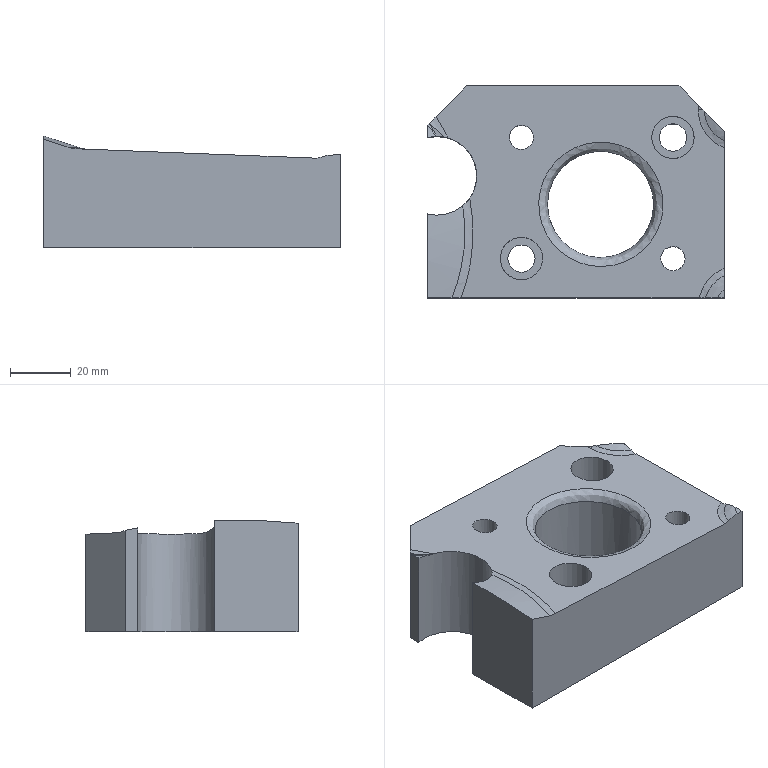Part | NX | features solid 2 | 1 solid | 31 faces | box 98.004 x 70.002 x 36.945 mm | volume 156458 mm3 | spline 13 | plane 10 | cylinder 8 | commonest cylinder face diameters 8 x2 9 x2 14 x2 26 x1 35.1 x1